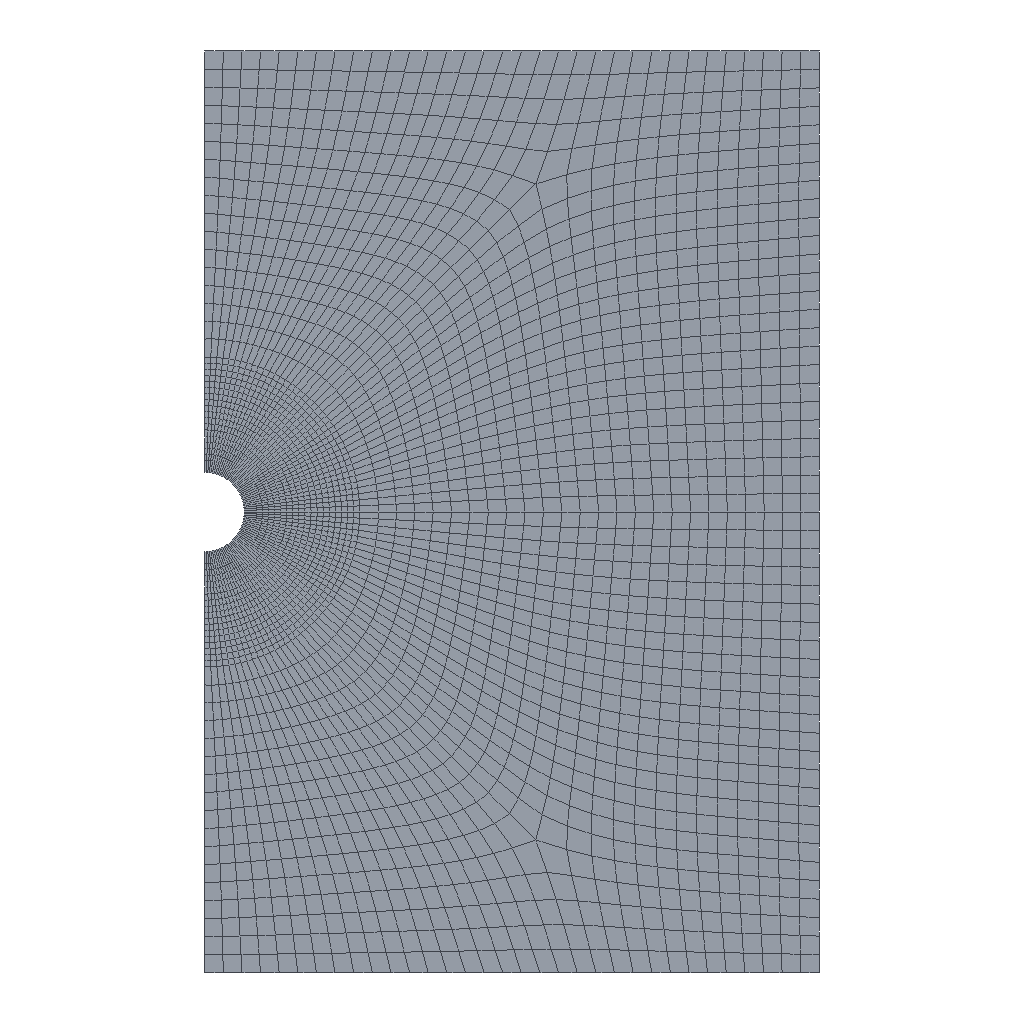Simulation study | abaqus
Set-up summary:
category,name,step,type,value,unit,region
solver,abaqus
solver,version,,,Abaqus/Standard 2020
units,not stated in the deck,,not stated
analysis,deck,,geostatic,geostatic
load_step,geo,geo,geostatic
load_step,Step-1,Step-1,soils
load_step,requested,,,2
mesh,nodes,,,3503
mesh,elements,,,3349
element_type,CPE4P,,plane,3330
element_type,COH2D4P,,cohesive,19
load,load commands in deck,,count,4
bc,support commands in deck,,count,5
material,COH,,in results
material,COH-0,,in results
material,ROCK,,in results
check,setup vs results,,match,"per instance, exact: element labels, types and connectivity; labels of the nodes the elements use; coordinates of those nodes at SINGLE_PRECISION in 1 of 1 instance(s)"
Abaqus input file, long lists of numbers shortened:
*Heading
** Job name: Job-1 Model name: Model-1-Copy
** Generated by: Abaqus/CAE 2020
*Preprint, echo=NO, model=NO, history=NO, contact=NO
**
** PARTS
**
*Part, name=work
*Node
      1,   25.206,           0.
      2,   6.441,           0.
** (3501 more lines like these left out)
*Element, type=CPE4P
  1,    1, 3466,  390,  125
  2, 3466, 3467,  391,  390
** (3328 more lines like these left out)
*Element, type=COH2D4P
3331,    1,   12, 3466,    1,    1, 3485
3332,   12,   13, 3467, 3466, 3485, 3486
** (17 more lines like these left out)
*Nset, nset=Set-111
    1,    2,    3,    4,    5,    6,   12,   13,   14,   15,   16,   17,   18,   19,   20,   21
   22,   23,   24,   25,   26,   27,   28,   29,   30,   31,   32,   33,   34,   35,   36,   37
** (101 more lines like these left out)
*Elset, elset=Set-111, generate
    1,  1520,     1
*Nset, nset=Set-120, generate
    1,  3484,     1
*Elset, elset=Set-120, generate
    1,  3330,     1
*Nset, nset=CohesiveSeam-2-TopNodes
    1, 3466, 3467, 3468, 3469, 3470, 3471, 3472, 3473, 3474, 3475, 3476, 3477, 3478, 3479, 3480
 3481, 3482, 3483, 3484
*Nset, nset=CohesiveSeam-2-BottomNodes
  1,  2, 12, 13, 14, 15, 16, 17, 18, 19, 20, 21, 22, 23, 24, 25
 26, 27, 28, 29
*Nset, nset=CohesiveSeam-2-MidNodes
    1, 3485, 3486, 3487, 3488, 3489, 3490, 3491, 3492, 3493, 3494, 3495, 3496, 3497, 3498, 3499
 3500, 3501, 3502, 3503
*Elset, elset=ele-3336-plug
 3336,
*Nset, nset=node-weiyi-0
   17, 3471, 3490
*Elset, elset=coh-shengyu
 3331, 3332, 3333, 3334, 3335, 3337, 3338, 3339, 3340, 3341, 3342, 3343, 3344, 3345, 3346, 3347
 3348, 3349
*Nset, nset=node-inject
 3503,
*Elset, elset=CohesiveSeam-2-Elements, generate
 3331,  3349,     1
*Elset, elset=Set-qilie
 3349,
*Elset, elset=Set-pore-pressure, generate
 775,  779,    1
*Elset, elset=pressure, generate
 10,  19,   1
*Nset, nset=Set-14
   12,   13,   14,   15,   16, 3466, 3467, 3468, 3469, 3470
*Nset, nset=Set-press
    2,   20,   21,   22,   23,   24,   25,   26,   27,   28,   29, 3474, 3475, 3476, 3477, 3478
 3479, 3480, 3481, 3482, 3483, 3484
*Elset, elset=__PickedSurf167_S3, internal, generate
 742,  760,    1
*Surface, type=ELEMENT, name=_PickedSurf167, internal
__PickedSurf167_S3, S3
*Elset, elset=__PickedSurf206_S3, internal, generate
 3331,  3349,     1
*Surface, type=ELEMENT, name=_PickedSurf206, internal
__PickedSurf206_S3, S3
*Elset, elset=_CohesiveSeam-2-TopSurf_S3, internal, generate
 3331,  3349,     1
*Surface, type=ELEMENT, name=CohesiveSeam-2-TopSurf
_CohesiveSeam-2-TopSurf_S3, S3
*Elset, elset=_CohesiveSeam-2-BottomSurf_S1, internal, generate
 3331,  3349,     1
*Surface, type=ELEMENT, name=CohesiveSeam-2-BottomSurf
_CohesiveSeam-2-BottomSurf_S1, S1
** Section: rock
*Solid Section, elset=Set-120, material=rock
,
** Section: coh
*Cohesive Section, elset=coh-shengyu, material=coh, response=TRACTION SEPARATION, thickness=SPECIFIED
0.001,
** Section: coh0
*Cohesive Section, elset=ele-3336-plug, material=coh-0, response=TRACTION SEPARATION, thickness=SPECIFIED
0.001,
*End Part
**
**
** ASSEMBLY
**
*Assembly, name=Assembly
**
*Instance, name=work-1, part=work
*Nset, nset=Set-14_PP_, internal
   12,   13,   14,   15,   16, 3466, 3467, 3468, 3469, 3470
*End Instance
**
*Nset, nset=Set-3, instance=work-1
   3,   4,   5,   6,  69,  70,  71,  72,  73,  74,  75,  76,  77,  78,  79,  80
  81,  82,  83,  84,  85,  86, 165, 166, 167, 168, 169, 170, 171, 172, 173, 174
** (1 more lines like these left out)
*Elset, elset=Set-3, instance=work-1
  742,  743,  744,  745,  746,  747,  748,  749,  750,  751,  752,  753,  754,  755,  756,  757
  758,  759,  760, 1502, 1503, 1504, 1505, 1506, 1507, 1508, 1509, 1510, 1511, 1512, 1513, 1514
** (1 more lines like these left out)
*Nset, nset=Set-4, instance=work-1
   7,   9, 222, 223, 224, 225, 226, 227, 228, 229, 230, 231, 232, 233, 234, 235
 236, 237, 238, 239, 240, 241, 242, 243, 244, 245
*Elset, elset=Set-4, instance=work-1
 1521, 1522, 1523, 1524, 1525, 1526, 1527, 1528, 1529, 1530, 1531, 1532, 1533, 1534, 1535, 1536
 1537, 1538, 1539, 1540, 2373, 2386, 2399, 2412, 2425
*Nset, nset=Set-5, instance=work-1
   8,   9, 286, 287, 288, 289, 290, 291, 292, 293, 294, 295, 296, 297, 298, 299
 300, 301, 302, 303, 304, 305, 306, 307, 308, 309, 310, 311, 312, 313, 314, 315
** (1 more lines like these left out)
*Elset, elset=Set-5, instance=work-1
 2265, 2270, 2275, 2280, 2285, 2290, 2295, 2300, 2305, 2310, 2315, 2320, 2325, 2330, 2335, 2340
 2345, 2350, 2355, 2360, 2361, 2362, 2363, 2364, 2365, 2366, 2367, 2368, 2369, 2370, 2371, 2372
** (1 more lines like these left out)
*Nset, nset=Set-12, instance=work-1
   7,   9, 222, 223, 224, 225, 226, 227, 228, 229, 230, 231, 232, 233, 234, 235
 236, 237, 238, 239, 240, 241, 242, 243, 244, 245
*Elset, elset=Set-12, instance=work-1
 1521, 1522, 1523, 1524, 1525, 1526, 1527, 1528, 1529, 1530, 1531, 1532, 1533, 1534, 1535, 1536
 1537, 1538, 1539, 1540, 2373, 2386, 2399, 2412, 2425
*Nset, nset=Set-13, instance=work-1
   8,   9, 286, 287, 288, 289, 290, 291, 292, 293, 294, 295, 296, 297, 298, 299
 300, 301, 302, 303, 304, 305, 306, 307, 308, 309, 310, 311, 312, 313, 314, 315
** (1 more lines like these left out)
*Elset, elset=Set-13, instance=work-1
 2265, 2270, 2275, 2280, 2285, 2290, 2295, 2300, 2305, 2310, 2315, 2320, 2325, 2330, 2335, 2340
 2345, 2350, 2355, 2360, 2361, 2362, 2363, 2364, 2365, 2366, 2367, 2368, 2369, 2370, 2371, 2372
** (1 more lines like these left out)
*Nset, nset=Set-14, instance=work-1
    1,    2,    3,    4,    5,    6,    7,    8,    9,   12,   13,   14,   15,   16,   17,   18
   19,   20,   21,   22,   23,   24,   25,   26,   27,   28,   29,   30,   31,   32,   33,   34
** (105 more lines like these left out)
*Elset, elset=Set-14, instance=work-1
    1,    2,    3,    4,    5,    6,    7,    8,    9,   10,   11,   12,   13,   14,   15,   16
   17,   18,   19,   20,   21,   22,   23,   24,   25,   26,   27,   28,   29,   30,   31,   32
** (97 more lines like these left out)
*Nset, nset=Set-15, instance=work-1
    1,    2,    3,    4,    5,    6,   12,   13,   14,   15,   16,   17,   18,   19,   20,   21
   22,   23,   24,   25,   26,   27,   28,   29,   30,   31,   32,   33,   34,   35,   36,   37
** (101 more lines like these left out)
*Elset, elset=Set-15, instance=work-1, generate
    1,  1520,     1
*Nset, nset=Set-16, instance=work-1
   3,   4,   5,   6,  69,  70,  71,  72,  73,  74,  75,  76,  77,  78,  79,  80
  81,  82,  83,  84,  85,  86, 165, 166, 167, 168, 169, 170, 171, 172, 173, 174
** (1 more lines like these left out)
*Elset, elset=Set-16, instance=work-1
  742,  743,  744,  745,  746,  747,  748,  749,  750,  751,  752,  753,  754,  755,  756,  757
  758,  759,  760, 1502, 1503, 1504, 1505, 1506, 1507, 1508, 1509, 1510, 1511, 1512, 1513, 1514
** (1 more lines like these left out)
*Nset, nset=Set-17, instance=work-1
    3,   30,   31,   32,   33,   34,   35,   36,   37,   38,   39,   40,   41,   42,   43,   44
   45,   46,   47,   48,   49,   50,   51,   52,   53,   54,   55,   56,   57,   58,   59,   60
** (1 more lines like these left out)
*Elset, elset=Set-17, instance=work-1, generate
  19,  760,   19
*Nset, nset=Set-18, instance=work-1
   3,   4,   5,   6,   8,  11,  69,  70,  71,  72,  73,  74,  75,  76,  77,  78
  79,  80,  81,  82,  83,  84,  85,  86, 165, 166, 167, 168, 169, 170, 171, 172
** (3 more lines like these left out)
*Elset, elset=Set-18, instance=work-1
  742,  743,  744,  745,  746,  747,  748,  749,  750,  751,  752,  753,  754,  755,  756,  757
  758,  759,  760, 1502, 1503, 1504, 1505, 1506, 1507, 1508, 1509, 1510, 1511, 1512, 1513, 1514
** (3 more lines like these left out)
*Nset, nset=Set-19, instance=work-1
   7,   9,  10, 222, 223, 224, 225, 226, 227, 228, 229, 230, 231, 232, 233, 234
 235, 236, 237, 238, 239, 240, 241, 242, 243, 244, 245, 318, 319, 320, 321, 322
** (2 more lines like these left out)
*Elset, elset=Set-19, instance=work-1
 1521, 1522, 1523, 1524, 1525, 1526, 1527, 1528, 1529, 1530, 1531, 1532, 1533, 1534, 1535, 1536
 1537, 1538, 1539, 1540, 2373, 2386, 2399, 2412, 2425, 2678, 2691, 2704, 2717, 2730, 2743, 2756
** (2 more lines like these left out)
*Nset, nset=Set-20, instance=work-1
   8,   9,  10,  11, 286, 287, 288, 289, 290, 291, 292, 293, 294, 295, 296, 297
 298, 299, 300, 301, 302, 303, 304, 305, 306, 307, 308, 309, 310, 311, 312, 313
** (3 more lines like these left out)
*Elset, elset=Set-20, instance=work-1
 2265, 2270, 2275, 2280, 2285, 2290, 2295, 2300, 2305, 2310, 2315, 2320, 2325, 2330, 2335, 2340
 2345, 2350, 2355, 2360, 2361, 2362, 2363, 2364, 2365, 2366, 2367, 2368, 2369, 2370, 2371, 2372
** (3 more lines like these left out)
*Nset, nset=Set-21, instance=work-1, generate
    1,  3484,     1
*Elset, elset=Set-21, instance=work-1, generate
    1,  3349,     1
*Nset, nset=Set-22, instance=work-1, generate
    1,  3484,     1
*Elset, elset=Set-22, instance=work-1, generate
    1,  3330,     1
*Elset, elset=_Surf-12_S2, internal, instance=work-1, generate
  19,  760,   19
*Surface, type=ELEMENT, name=Surf-12
_Surf-12_S2, S2
*Elset, elset=_Surf-14_S2, internal, instance=work-1, generate
  19,  760,   19
*Elset, elset=_Surf-14_S4, internal, instance=work-1, generate
  761,  1502,    19
*Surface, type=ELEMENT, name=Surf-14
_Surf-14_S2, S2
_Surf-14_S4, S4
*End Assembly
*Amplitude, name=Amp-1
             0.,              0.,             50.,              1.
**
** MATERIALS
**
*Material, name=coh
*Damage Initiation, criterion=MAXS
 1e+06,  5e+06,500000.
*Damage Evolution, type=DISPLACEMENT
 1e-09,
*Elastic, type=TRACTION
 1.5e+10, 1.5e+10, 1.5e+10
*Fluid Leakoff
 1e-14, 1e-14
*Gap Flow
 0.001,
*Material, name=coh-0
*Damage Initiation, criterion=MAXS
 1e+06, 5e+06, 5e+06
*Damage Evolution, type=DISPLACEMENT
 1e-09,
*Elastic, type=TRACTION
 1.5e+10, 1.5e+10, 1.5e+10
*Gap Flow
 1e-50,
*Material, name=rock
*Elastic
 1.5e+10, 0.25
*Permeability, specific=9800.
 1e-07, 0.2
**
** INTERACTION PROPERTIES
**
*Surface Interaction, name=IntProp-1
1.,
**
** BOUNDARY CONDITIONS
**
** Name: [REDACTED] : Displacement/rotation angle
*Boundary
work-1.node-weiyi-0, 2, 2
** Name: [REDACTED] : Displacement/rotation angle
*Boundary
Set-19, 1, 1
** Name: [REDACTED] : Symmetric / antisymmetric / fully fixed
*Boundary
Set-18, XSYMM
** Name: [REDACTED] : Displacement/rotation angle
*Boundary
Set-20, 2, 2
**
** PREDEFINED FIELDS
**
** Name: Predefined Field-1   Type: Void ratio
*Initial Conditions, TYPE=RATIO
Set-21, 0.2
** Name: Predefined Field-2   Type: Stress
*Initial Conditions, type=STRESS
Set-22, -1e+06, -1e+06, -1e+06, 0.,
** ----------------------------------------------------------------
*initial conditions,type=initial gap
work-1.Set-qilie
**
** STEP: geo
**
*Step, name=geo, nlgeom=NO, unsymm=YES
*Geostatic
**
** CONTROLS
**
*Controls, reset
*Controls, parameters=time incrementation
, , , , , , , 20, , ,
**
** OUTPUT REQUESTS
**
*Restart, write, frequency=0
**
** FIELD OUTPUT: F-Output-1
**
*Output, field
*Node Output
CF, PHILSM, POR, PSILSM, RF, U
*Element Output, directions=YES
E, FLUVR, FLVEL, LE, LOADSXFEM, MISES, PFOPENXFEM, S, SAT, SDEG, VOIDR,pfopen
*Contact Output
CSDMG, PFL, PFLA, PTL, PTLA
*Output, history, frequency=0
*End Step
** ----------------------------------------------------------------
**
** STEP: Step-1
**
*Step, name=Step-1, nlgeom=YES, inc=10000, unsymm=YES
*Soils, consolidation, end=PERIOD, utol=1e+25, creep=none
0.01, 50., 3e-06, 50.,
**
** BOUNDARY CONDITIONS
**
** Name: BC-5 Type: 孔隙压力
*Boundary, amplitude=Amp-1
work-1.Set-14_PP_, 8, 8, 100000.
**
** LOADS
**
** Name: Load-2   Type: Pressure
*Dsload, amplitude=Amp-1
Surf-14, P, 1000.
** Name: Load-3   Type: Concentrated pore fluid
*Cflow, amplitude=Amp-1
work-1.node-inject,  , -0.005
** Name: Load-4   Type: Concentrated force
*Cload, amplitude=Amp-1
work-1.Set-press, 2, -1000.
**
** CONTROLS
**
*Controls, reset
*Controls, parameters=time incrementation
, , , , , , , 20, , ,
**
** OUTPUT REQUESTS
**
*Restart, write, frequency=0
**
** FIELD OUTPUT: F-Output-1
**
*Output, field
*Node Output
CF, PHILSM, POR, PSILSM, RF, U
*Element Output, directions=YES
E, FLUVR, FLVEL, LE, MISES, S, SAT, SDEG, VOIDR,pfopen
*Contact Output
CSDMG, PFL, PFLA, PTL, PTLA
**
** HISTORY OUTPUT: H-Output-1
**
*Output, history
*Node Output, nset=work-1.node-inject
POR,
*End Step
Results summary:
result,step,,completed,increments=1 time=1.0/1.0
result,step,,completed,increments=30 time=50.0/50.0
result,analysis,,,"soils, consolidation"
result,last_loadstep,,,2
result,primary field,,,"U, POR"
result,reaction total,,FX,-12861.0,model units
result,reaction total,,FY,21986.0,model units
result,reaction total,,FZ,0.0,model units